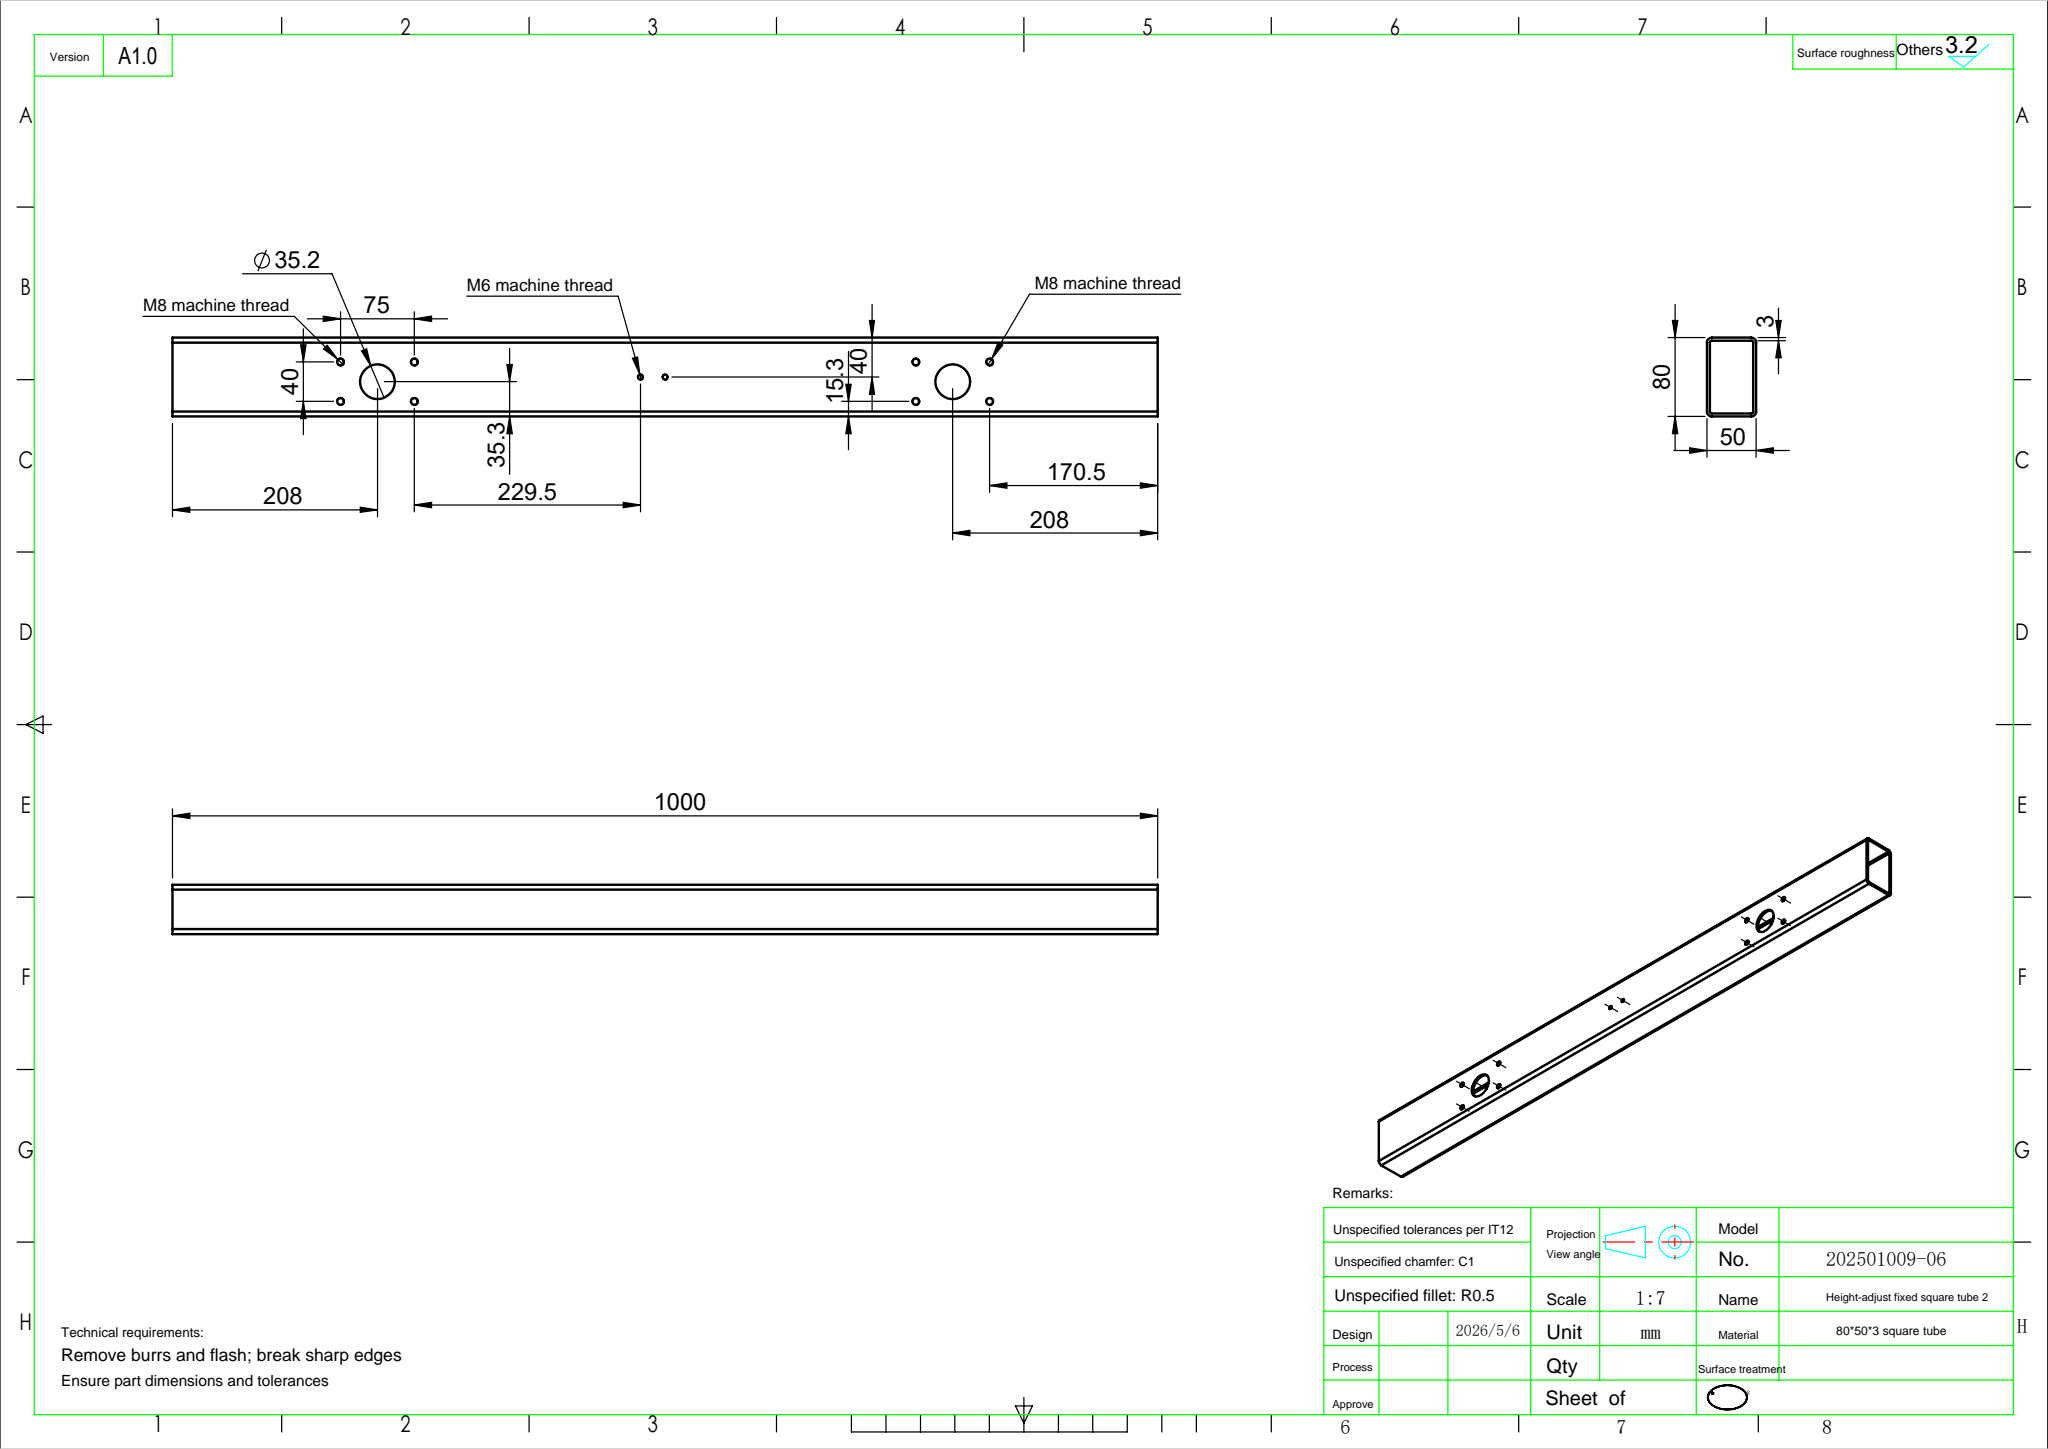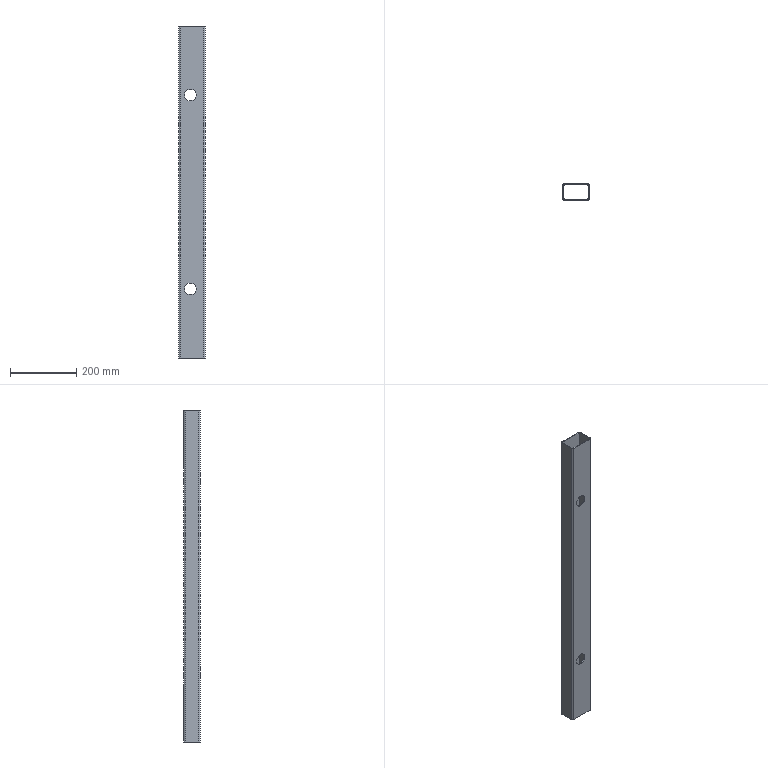Part | SolidWorks | features ICE 2, Cut 1, Extrusion 1, Fillet 1, Shell 1 | 1 solid | 46 faces | box 80 x 50 x 1000 mm | volume 713306 mm3 | cylinder 36 | plane 10 | commonest cylinder face diameters 6.8 x16 35.2 x8 4 x4 5 x4 10 x4